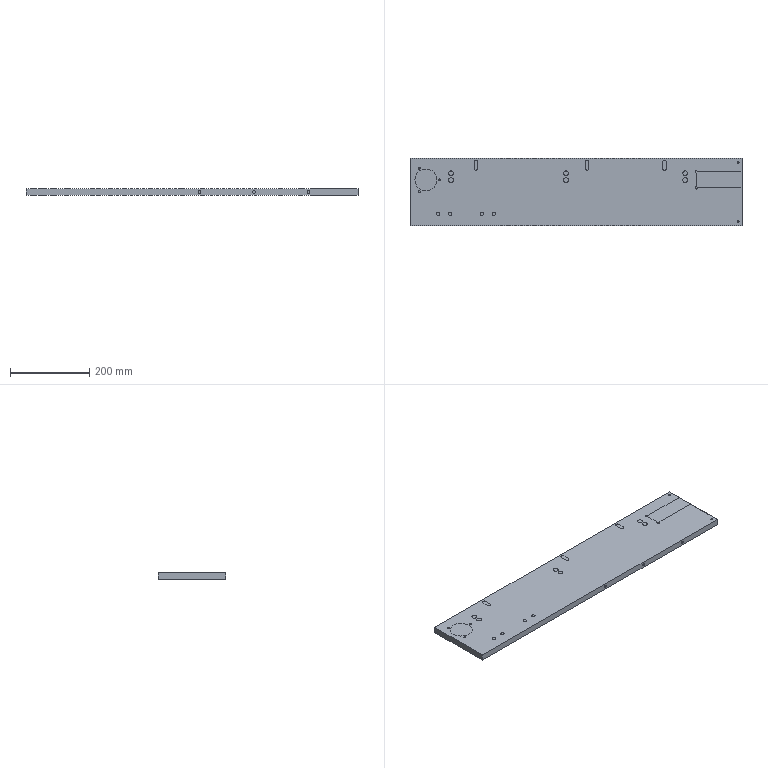NC program | NX | posted with a generic post | part box 836 x 170 x 16 mm
Lines 1 to 237 of 11551:
N10 G17 G21 G94 G90
(G81点孔 , TOOL : D6点孔钻)
N12 T01 M6
N14 /M1
N16 G54
N18 G17 G0 G90 X103. Y132. S1500 M3
N20 G43 Z100. H1
N22 G94 G81 G98 Z-1.5 F100. R1.5
N24 Y115.
N26 X74. Y115.5
N28 X23. Y144.945
N30 X40. Y115.5
N32 X23. Y86.055
N34 X71. Y30.
N36 X101.
N38 X181.
N40 X211.
N42 X393. Y115.
N44 Y132.
N46 X693. Y115.
N48 Y132.
N50 X826. Y160.
N52 Y10.
N54 G80
N56 G0 X826. Y10. Z100.
N58 M5
(孔铣开粗_2 , TOOL : D17R0.8圆鼻飞刀)
N60 T14 M6
N62 /M1
N64 G54
N66 G17 G0 G90 X40. Y115.5 S2000 M3
N68 G43 Z100. H14
N70 Z1.2
N72 G94 G1 Z0.2 F1040.
N74 G3 X44. Y111.5 R4.
N76 X48. Y115.5 R4.
N78 X48. Y115.5 Z0. I-8. J0. F1300.
N80 X48. Y115.5 Z-0.2 I-8. J0.
N82 X48. Y115.5 Z-0.4 I-8. J0.
N84 X48. Y115.5 Z-0.6 I-8. J0.
N86 X48. Y115.5 Z-0.8 I-8. J0.
N88 X48. Y115.5 Z-1. I-8. J0.
N90 X48. Y115.5 Z-1.2 I-8. J0.
N92 X48. Y115.5 Z-1.4 I-8. J0.
N94 X48. Y115.5 Z-1.6 I-8. J0.
N96 X48. Y115.5 Z-1.8 I-8. J0.
N98 X48. Y115.5 Z-2. I-8. J0.
N100 X48. Y115.5 Z-2.2 I-8. J0.
N102 X48. Y115.5 Z-2.4 I-8. J0.
N104 X48. Y115.5 Z-2.6 I-8. J0.
N106 X48. Y115.5 Z-2.8 I-8. J0.
N108 X48. Y115.5 Z-3. I-8. J0.
N110 X48. Y115.5 Z-3.2 I-8. J0.
N112 X48. Y115.5 Z-3.4 I-8. J0.
N114 X48. Y115.5 Z-3.6 I-8. J0.
N116 X48. Y115.5 Z-3.8 I-8. J0.
N118 X48. Y115.5 Z-4. I-8. J0.
N120 X48. Y115.5 Z-4.2 I-8. J0.
N122 X48. Y115.5 Z-4.4 I-8. J0.
N124 X48. Y115.5 Z-4.6 I-8. J0.
N126 X48. Y115.5 Z-4.8 I-8. J0.
N128 X48. Y115.5 Z-5. I-8. J0.
N130 X48. Y115.5 Z-5.2 I-8. J0.
N132 X48. Y115.5 Z-5.4 I-8. J0.
N134 X48. Y115.5 Z-5.6 I-8. J0.
N136 X48. Y115.5 Z-5.8 I-8. J0.
N138 X48. Y115.5 Z-6. I-8. J0.
N140 X48. Y115.5 Z-6.2 I-8. J0.
N142 X48. Y115.5 Z-6.4 I-8. J0.
N144 X48. Y115.5 Z-6.6 I-8. J0.
N146 X48. Y115.5 Z-6.8 I-8. J0.
N148 X48. Y115.5 Z-7. I-8. J0.
N150 X48. Y115.5 Z-7.2 I-8. J0.
N152 X48. Y115.5 Z-7.4 I-8. J0.
N154 X48. Y115.5 Z-7.6 I-8. J0.
N156 X48. Y115.5 Z-7.8 I-8. J0.
N158 X48. Y115.5 Z-8. I-8. J0.
N160 X48. Y115.5 Z-8.2 I-8. J0.
N162 X48. Y115.5 Z-8.4 I-8. J0.
N164 X48. Y115.5 Z-8.6 I-8. J0.
N166 X48. Y115.5 Z-8.8 I-8. J0.
N168 X48. Y115.5 Z-9. I-8. J0.
N170 X48. Y115.5 Z-9.2 I-8. J0.
N172 X48. Y115.5 Z-9.4 I-8. J0.
N174 X48. Y115.5 Z-9.6 I-8. J0.
N176 X48. Y115.5 Z-9.8 I-8. J0.
N178 X48. Y115.5 Z-10. I-8. J0.
N180 X48. Y115.5 Z-10.2 I-8. J0.
N182 X48. Y115.5 Z-10.4 I-8. J0.
N184 X48. Y115.5 Z-10.6 I-8. J0.
N186 X48. Y115.5 Z-10.8 I-8. J0.
N188 X48. Y115.5 Z-11. I-8. J0.
N190 X48. Y115.5 Z-11.2 I-8. J0.
N192 X48. Y115.5 Z-11.4 I-8. J0.
N194 X48. Y115.5 Z-11.6 I-8. J0.
N196 X48. Y115.5 Z-11.8 I-8. J0.
N198 X48. Y115.5 Z-12. I-8. J0.
N200 X48. Y115.5 Z-12.2 I-8. J0.
N202 X48. Y115.5 Z-12.4 I-8. J0.
N204 X48. Y115.5 Z-12.6 I-8. J0.
N206 X48. Y115.5 Z-12.8 I-8. J0.
N208 X48. Y115.5 Z-13. I-8. J0.
N210 X48. Y115.5 Z-13.2 I-8. J0.
N212 X48. Y115.5 Z-13.4 I-8. J0.
N214 X48. Y115.5 Z-13.6 I-8. J0.
N216 X48. Y115.5 Z-13.8 I-8. J0.
N218 X48. Y115.5 Z-14. I-8. J0.
N220 X48. Y115.5 Z-14.2 I-8. J0.
N222 X48. Y115.5 Z-14.4 I-8. J0.
N224 X48. Y115.5 Z-14.6 I-8. J0.
N226 X48. Y115.5 Z-14.8 I-8. J0.
N228 X48. Y115.5 Z-15. I-8. J0.
N230 X48. Y115.5 Z-15.2 I-8. J0.
N232 X48. Y115.5 Z-15.4 I-8. J0.
N234 X48. Y115.5 Z-15.6 I-8. J0.
N236 X48. Y115.5 Z-15.8 I-8. J0.
N238 X48. Y115.5 Z-16. I-8. J0.
N240 X48. Y115.5 Z-16.2 I-8. J0.
N242 X48. Y115.5 Z-16.4 I-8. J0.
N244 X48. Y115.5 Z-16.6 I-8. J0.
N246 X48. Y115.5 Z-16.8 I-8. J0.
N248 X48. Y115.5 Z-17. I-8. J0.
N250 X40. Y123.5 R8.
N252 X48. Y115.5 R-8.
N254 X44. Y119.5 R4.
N256 X40. Y115.5 R4.
N258 G0 Z100.
N260 M5
(#### , TOOL : D21R0.8####)
N262 T09 M6
N264 /M1
N266 G54
N268 G17 G0 G90 X40. Y115.5 S1700 M3
N270 G43 Z100. H9
N272 Z1.2
N274 G94 G1 Z0.2 F1200.
N276 X40.135 Y114.509
N278 G3 X54.8 Y115.5 R7.366
N280 X54.8 Y115.5 Z0. I-14.8 J0. F1500.
N282 X54.8 Y115.5 Z-0.2 I-14.8 J0.
N284 X54.8 Y115.5 Z-0.4 I-14.8 J0.
N286 X54.8 Y115.5 Z-0.6 I-14.8 J0.
N288 X54.8 Y115.5 Z-0.8 I-14.8 J0.
N290 X54.8 Y115.5 Z-1. I-14.8 J0.
N292 X54.8 Y115.5 Z-1.2 I-14.8 J0.
N294 X54.8 Y115.5 Z-1.4 I-14.8 J0.
N296 X54.8 Y115.5 Z-1.6 I-14.8 J0.
N298 X54.8 Y115.5 Z-1.8 I-14.8 J0.
N300 X54.8 Y115.5 Z-2. I-14.8 J0.
N302 X54.8 Y115.5 Z-2.2 I-14.8 J0.
N304 X54.8 Y115.5 Z-2.4 I-14.8 J0.
N306 X54.8 Y115.5 Z-2.6 I-14.8 J0.
N308 X54.8 Y115.5 Z-2.8 I-14.8 J0.
N310 X54.8 Y115.5 Z-3. I-14.8 J0.
N312 X54.8 Y115.5 Z-3.2 I-14.8 J0.
N314 X54.8 Y115.5 Z-3.4 I-14.8 J0.
N316 X54.8 Y115.5 Z-3.6 I-14.8 J0.
N318 X54.8 Y115.5 Z-3.8 I-14.8 J0.
N320 X54.8 Y115.5 Z-4. I-14.8 J0.
N322 X54.8 Y115.5 Z-4.2 I-14.8 J0.
N324 X54.8 Y115.5 Z-4.4 I-14.8 J0.
N326 X54.8 Y115.5 Z-4.6 I-14.8 J0.
N328 X54.8 Y115.5 Z-4.8 I-14.8 J0.
N330 X54.8 Y115.5 Z-5. I-14.8 J0.
N332 X54.8 Y115.5 Z-5.2 I-14.8 J0.
N334 X54.8 Y115.5 Z-5.4 I-14.8 J0.
N336 X54.8 Y115.5 Z-5.6 I-14.8 J0.
N338 X54.8 Y115.5 Z-5.8 I-14.8 J0.
N340 X54.8 Y115.5 Z-6. I-14.8 J0.
N342 X54.8 Y115.5 Z-6.2 I-14.8 J0.
N344 X54.8 Y115.5 Z-6.4 I-14.8 J0.
N346 X54.8 Y115.5 Z-6.6 I-14.8 J0.
N348 X54.8 Y115.5 Z-6.8 I-14.8 J0.
N350 X54.8 Y115.5 Z-7. I-14.8 J0.
N352 X54.8 Y115.5 Z-7.2 I-14.8 J0.
N354 X54.8 Y115.5 Z-7.4 I-14.8 J0.
N356 X54.8 Y115.5 Z-7.6 I-14.8 J0.
N358 X54.8 Y115.5 Z-7.8 I-14.8 J0.
N360 X54.8 Y115.5 Z-8. I-14.8 J0.
N362 X54.8 Y115.5 Z-8.2 I-14.8 J0.
N364 X54.8 Y115.5 Z-8.4 I-14.8 J0.
N366 X54.8 Y115.5 Z-8.6 I-14.8 J0.
N368 X54.8 Y115.5 Z-8.8 I-14.8 J0.
N370 X54.8 Y115.5 Z-9. I-14.8 J0.
N372 X54.8 Y115.5 Z-9.2 I-14.8 J0.
N374 X54.8 Y115.5 Z-9.4 I-14.8 J0.
N376 X54.8 Y115.5 Z-9.6 I-14.8 J0.
N378 X54.8 Y115.5 Z-9.8 I-14.8 J0.
N380 X54.8 Y115.5 Z-10. I-14.8 J0.
N382 X54.8 Y115.5 Z-10.2 I-14.8 J0.
N384 X54.8 Y115.5 Z-10.4 I-14.8 J0.
N386 X54.8 Y115.5 Z-10.6 I-14.8 J0.
N388 X54.8 Y115.5 Z-10.8 I-14.8 J0.
N390 X54.8 Y115.5 Z-11. I-14.8 J0.
N392 X54.8 Y115.5 Z-11.2 I-14.8 J0.
N394 X54.8 Y115.5 Z-11.4 I-14.8 J0.
N396 X54.8 Y115.5 Z-11.6 I-14.8 J0.
N398 X54.8 Y115.5 Z-11.8 I-14.8 J0.
N400 X54.8 Y115.5 Z-12. I-14.8 J0.
N402 X54.8 Y115.5 Z-12.2 I-14.8 J0.
N404 X54.8 Y115.5 Z-12.4 I-14.8 J0.
N406 X54.8 Y115.5 Z-12.6 I-14.8 J0.
N408 X54.8 Y115.5 Z-12.8 I-14.8 J0.
N410 X54.8 Y115.5 Z-13. I-14.8 J0.
N412 X54.8 Y115.5 Z-13.2 I-14.8 J0.
N414 X54.8 Y115.5 Z-13.4 I-14.8 J0.
N416 X54.8 Y115.5 Z-13.6 I-14.8 J0.
N418 X54.8 Y115.5 Z-13.8 I-14.8 J0.
N420 X54.8 Y115.5 Z-14. I-14.8 J0.
N422 X54.8 Y115.5 Z-14.2 I-14.8 J0.
N424 X54.8 Y115.5 Z-14.4 I-14.8 J0.
N426 X54.8 Y115.5 Z-14.6 I-14.8 J0.
N428 X54.8 Y115.5 Z-14.8 I-14.8 J0.
N430 X54.8 Y115.5 Z-15. I-14.8 J0.
N432 X54.8 Y115.5 Z-15.2 I-14.8 J0.
N434 X54.8 Y115.5 Z-15.4 I-14.8 J0.
N436 X54.8 Y115.5 Z-15.6 I-14.8 J0.
N438 X54.8 Y115.5 Z-15.8 I-14.8 J0.
N440 X54.8 Y115.5 Z-16. I-14.8 J0.
N442 X54.8 Y115.5 Z-16.2 I-14.8 J0.
N444 X54.8 Y115.5 Z-16.4 I-14.8 J0.
N446 X54.8 Y115.5 Z-16.6 I-14.8 J0.
N448 X54.8 Y115.5 Z-16.8 I-14.8 J0.
N450 X54.8 Y115.5 Z-17. I-14.8 J0.
N452 X40. Y130.3 R14.8
N454 X54.8 Y115.5 R-14.8
N456 X40.135 Y116.491 R7.366
N458 G1 X40. Y115.5
N460 G0 Z100.